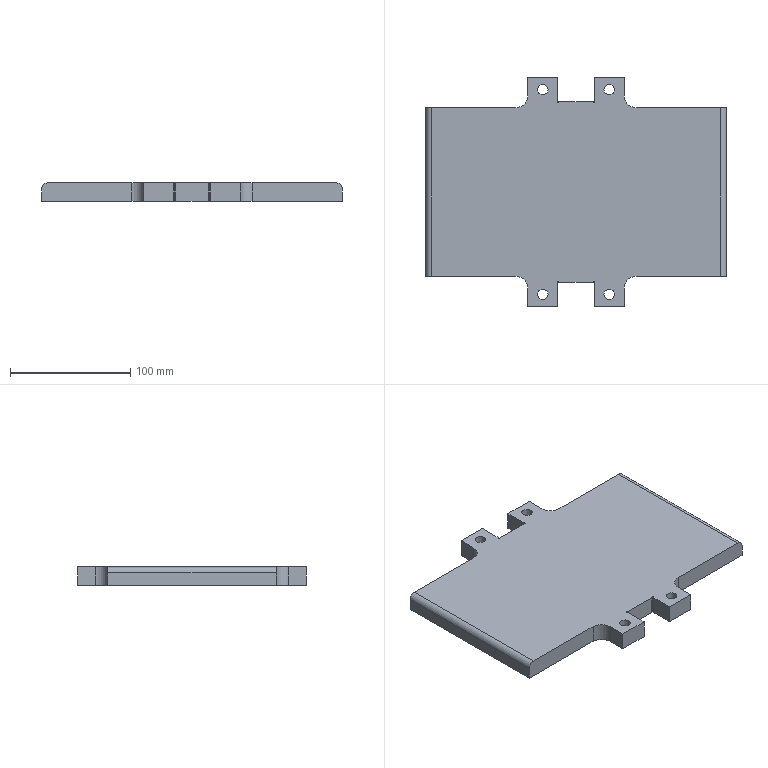Part | STEP file | YBQDJ-YY-4 | 1 solid | 44 faces | box 250 x 190 x 15 mm | volume 563148 mm3 | plane 22 | cylinder 22 | commonest cylinder face diameters 4 x8 1 x4 8.7 x4 20 x4 10 x2